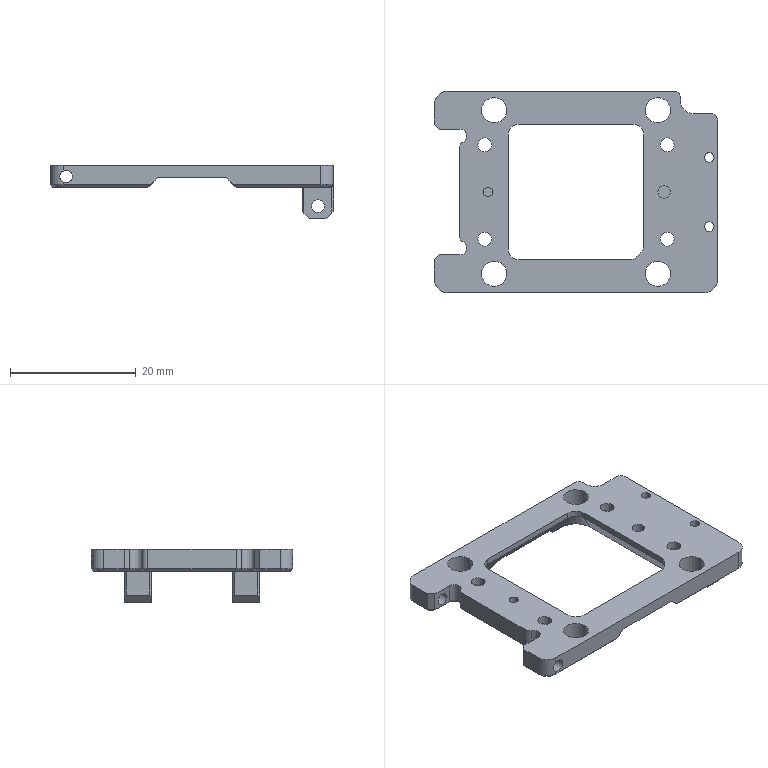NC program | NX | posted with a generic post | part box 45 x 32 x 8.5 mm
Lines 869 to 3036 of 3806, first 1647 of 2162 lines:
(CAVITY_MILL , TOOL : D3)
N1706 T17 M6
N1708 G54
N1710 G17 G0 G90 X18.406 Y16.355 B0. C0. S9500 M3
N1712 G43 Z30. H17
N1714 Z0.722
N1716 G94 G1 Z-0.278 F1100.
N1718 G3 X18.08 Y15.431 R1.
N1720 G2 X18.118 Y15. R2.5
N1722 G1 Y14.437
N1724 G3 X18.618 Y13.937 R0.5
N1726 G1 X19.665
N1728 G3 X20.531 Y14.437 R1.
N1730 G1 X20.589 Y14.537
N1732 Z0.722
N1734 G0 Z30.
N1736 X18.406 Y16.355
N1738 Z0.444
N1740 G1 Z-0.556
N1742 G3 X18.08 Y15.431 R1.
N1744 G2 X18.118 Y15. R2.5
N1746 G1 Y14.437
N1748 G3 X18.618 Y13.937 R0.5
N1750 G1 X19.665
N1752 G3 X20.531 Y14.437 R1.
N1754 G1 X20.589 Y14.537
N1756 Z0.444
N1758 G0 Z30.
N1760 X18.406 Y16.355
N1762 Z0.167
N1764 G1 Z-0.833
N1766 G3 X18.08 Y15.431 R1.
N1768 G2 X18.118 Y15. R2.5
N1770 G1 Y14.437
N1772 G3 X18.618 Y13.937 R0.5
N1774 G1 X19.665
N1776 G3 X20.531 Y14.437 R1.
N1778 G1 X20.589 Y14.537
N1780 Z0.167
N1782 G0 X18.406 Y16.355 Z-0.111
N1784 G1 Z-1.111
N1786 G3 X18.08 Y15.431 R1.
N1788 G2 X18.118 Y15. R2.5
N1790 G1 Y14.437
N1792 G3 X18.618 Y13.937 R0.5
N1794 G1 X19.665
N1796 G3 X20.531 Y14.437 R1.
N1798 G1 X20.589 Y14.537
N1800 Z-0.111
N1802 G0 X18.406 Y16.355 Z-0.389
N1804 G1 Z-1.389
N1806 G3 X18.08 Y15.431 R1.
N1808 G2 X18.118 Y15. R2.5
N1810 G1 Y14.437
N1812 G3 X18.618 Y13.937 R0.5
N1814 G1 X19.665
N1816 G3 X20.531 Y14.437 R1.
N1818 G1 X20.589 Y14.537
N1820 Z-0.389
N1822 G0 X18.406 Y16.355 Z-0.667
N1824 G1 Z-1.667
N1826 G3 X18.08 Y15.431 R1.
N1828 G2 X18.118 Y15. R2.5
N1830 G1 Y14.437
N1832 G3 X18.618 Y13.937 R0.5
N1834 G1 X19.665
N1836 G3 X20.531 Y14.437 R1.
N1838 G1 X20.589 Y14.537
N1840 Z-0.667
N1842 G0 X18.406 Y16.355 Z-0.944
N1844 G1 Z-1.944
N1846 G3 X18.08 Y15.431 R1.
N1848 G2 X18.118 Y15. R2.5
N1850 G1 Y14.437
N1852 G3 X18.618 Y13.937 R0.5
N1854 G1 X19.665
N1856 G3 X20.531 Y14.437 R1.
N1858 G1 X20.589 Y14.537
N1860 Z-0.944
N1862 G0 X18.406 Y16.355 Z-1.222
N1864 G1 Z-2.222
N1866 G3 X18.08 Y15.431 R1.
N1868 G2 X18.118 Y15. R2.5
N1870 G1 Y14.437
N1872 G3 X18.618 Y13.937 R0.5
N1874 G1 X19.665
N1876 G3 X20.531 Y14.437 R1.
N1878 G1 X20.589 Y14.537
N1880 Z-1.222
N1882 G0 X18.406 Y16.355 Z-1.5
N1884 G1 Z-2.5
N1886 G3 X18.08 Y15.431 R1.
N1888 G2 X18.118 Y15. R2.5
N1890 G1 Y14.437
N1892 G3 X18.618 Y13.937 R0.5
N1894 G1 X19.665
N1896 G3 X20.531 Y14.437 R1.
N1898 G1 X20.589 Y14.537
N1900 Z-1.5
N1902 G0 X18.406 Y16.355 Z-1.8
N1904 G1 Z-2.8
N1906 G3 X18.08 Y15.431 R1.
N1908 G2 X18.118 Y15. R2.5
N1910 G1 Y14.437
N1912 G3 X18.618 Y13.937 R0.5
N1914 G1 X19.665
N1916 G3 X20.531 Y14.437 R1.
N1918 G1 X20.589 Y14.537
N1920 Z-1.8
N1922 G0 X18.406 Y16.355 Z-2.1
N1924 G1 Z-3.1
N1926 G3 X18.08 Y15.431 R1.
N1928 G2 X18.118 Y15. R2.5
N1930 G1 Y14.437
N1932 G3 X18.618 Y13.937 R0.5
N1934 G1 X19.665
N1936 G3 X20.531 Y14.437 R1.
N1938 G1 X20.589 Y14.537
N1940 Z-2.1
N1942 G0 X18.402 Y16.362 Z-2.4
N1944 G1 Z-3.4
N1946 G3 X18.079 Y15.437 R1.
N1948 G2 X18.118 Y15. R2.5
N1950 G1 Y14.437
N1952 G3 X18.618 Y13.937 R0.5
N1954 G1 X19.699
N1956 G3 X20.565 Y14.437 R1.
N1958 G1 X20.623 Y14.537
N1960 Z-2.4
N1962 G0 X18.402 Y16.362 Z-2.7
N1964 G1 Z-3.7
N1966 G3 X18.079 Y15.437 R1.
N1968 G2 X18.118 Y15. R2.5
N1970 G1 Y14.437
N1972 G3 X18.618 Y13.937 R0.5
N1974 G1 X19.699
N1976 G3 X20.565 Y14.437 R1.
N1978 G1 X20.623 Y14.537
N1980 Z-2.7
N1982 G0 X18.402 Y16.362 Z-3.
N1984 G1 Z-4.
N1986 G3 X18.079 Y15.437 R1.
N1988 G2 X18.118 Y15. R2.5
N1990 G1 Y14.437
N1992 G3 X18.618 Y13.937 R0.5
N1994 G1 X19.699
N1996 G3 X20.565 Y14.437 R1.
N1998 G1 X20.623 Y14.537
N2000 Z-3.
N2002 G0 X18.402 Y16.362 Z-3.3
N2004 G1 Z-4.3
N2006 G3 X18.079 Y15.437 R1.
N2008 G2 X18.118 Y15. R2.5
N2010 G1 Y14.437
N2012 G3 X18.618 Y13.937 R0.5
N2014 G1 X19.699
N2016 G3 X20.565 Y14.437 R1.
N2018 G1 X20.623 Y14.537
N2020 Z-3.3
N2022 G0 X18.402 Y16.362 Z-3.6
N2024 G1 Z-4.6
N2026 G3 X18.079 Y15.437 R1.
N2028 G2 X18.118 Y15. R2.5
N2030 G1 Y14.437
N2032 G3 X18.618 Y13.937 R0.5
N2034 G1 X19.699
N2036 G3 X20.565 Y14.437 R1.
N2038 G1 X20.623 Y14.537
N2040 Z-3.6
N2042 G0 X18.402 Y16.362 Z-3.9
N2044 G1 Z-4.9
N2046 G3 X18.079 Y15.437 R1.
N2048 G2 X18.118 Y15. R2.5
N2050 G1 Y14.437
N2052 G3 X18.618 Y13.937 R0.5
N2054 G1 X19.699
N2056 G3 X20.565 Y14.437 R1.
N2058 G1 X20.623 Y14.537
N2060 Z-3.9
N2062 G0 X18.402 Y16.362 Z-4.2
N2064 G1 Z-5.2
N2066 G3 X18.079 Y15.437 R1.
N2068 G2 X18.118 Y15. R2.5
N2070 G1 Y14.437
N2072 G3 X18.618 Y13.937 R0.5
N2074 G1 X19.699
N2076 G3 X20.565 Y14.437 R1.
N2078 G1 X20.623 Y14.537
N2080 Z-4.2
N2082 G0 X18.402 Y16.362 Z-4.5
N2084 G1 Z-5.5
N2086 G3 X18.079 Y15.437 R1.
N2088 G2 X18.118 Y15. R2.5
N2090 G1 Y14.437
N2092 G3 X18.618 Y13.937 R0.5
N2094 G1 X19.699
N2096 G3 X20.565 Y14.437 R1.
N2098 G1 X20.623 Y14.537
N2100 Z-4.5
N2102 G0 X18.402 Y16.362 Z-4.8
N2104 G1 Z-5.8
N2106 G3 X18.079 Y15.437 R1.
N2108 G2 X18.118 Y15. R2.5
N2110 G1 Y14.437
N2112 G3 X18.618 Y13.937 R0.5
N2114 G1 X19.699
N2116 G3 X20.565 Y14.437 R1.
N2118 G1 X20.623 Y14.537
N2120 Z-4.8
N2122 G0 X18.402 Y16.362 Z-5.1
N2124 G1 Z-6.1
N2126 G3 X18.079 Y15.437 R1.
N2128 G2 X18.118 Y15. R2.5
N2130 G1 Y14.437
N2132 G3 X18.618 Y13.937 R0.5
N2134 G1 X19.699
N2136 G3 X20.565 Y14.437 R1.
N2138 G1 X20.623 Y14.537
N2140 Z-5.1
N2142 G0 X18.402 Y16.362 Z-5.4
N2144 G1 Z-6.4
N2146 G3 X18.079 Y15.437 R1.
N2148 G2 X18.118 Y15. R2.5
N2150 G1 Y14.437
N2152 G3 X18.618 Y13.937 R0.5
N2154 G1 X19.699
N2156 G3 X20.565 Y14.437 R1.
N2158 G1 X20.623 Y14.537
N2160 Z-5.4
N2162 G0 X18.402 Y16.362 Z-5.7
N2164 G1 Z-6.7
N2166 G3 X18.079 Y15.437 R1.
N2168 G2 X18.118 Y15. R2.5
N2170 G1 Y14.437
N2172 G3 X18.618 Y13.937 R0.5
N2174 G1 X19.699
N2176 G3 X20.565 Y14.437 R1.
N2178 G1 X20.623 Y14.537
N2180 Z-5.7
N2182 G0 X18.402 Y16.362 Z-6.
N2184 G1 Z-7.
N2186 G3 X18.079 Y15.437 R1.
N2188 G2 X18.118 Y15. R2.5
N2190 G1 Y14.437
N2192 G3 X18.618 Y13.937 R0.5
N2194 G1 X19.699
N2196 G3 X20.565 Y14.437 R1.
N2198 G1 X20.623 Y14.537
N2200 Z-6.
N2202 G0 X18.402 Y16.362 Z-6.3
N2204 G1 Z-7.3
N2206 G3 X18.079 Y15.437 R1.
N2208 G2 X18.118 Y15. R2.5
N2210 G1 Y14.437
N2212 G3 X18.618 Y13.937 R0.5
N2214 G1 X19.699
N2216 G3 X20.565 Y14.437 R1.
N2218 G1 X20.623 Y14.537
N2220 Z-6.3
N2222 G0 X18.402 Y16.362 Z-6.6
N2224 G1 Z-7.6
N2226 G3 X18.079 Y15.437 R1.
N2228 G2 X18.118 Y15. R2.5
N2230 G1 Y14.437
N2232 G3 X18.618 Y13.937 R0.5
N2234 G1 X19.699
N2236 G3 X20.565 Y14.437 R1.
N2238 G1 X20.623 Y14.537
N2240 Z-6.6
N2242 G0 X18.402 Y16.362 Z-6.9
N2244 G1 Z-7.9
N2246 G3 X18.079 Y15.437 R1.
N2248 G2 X18.118 Y15. R2.5
N2250 G1 Y14.437
N2252 G3 X18.618 Y13.937 R0.5
N2254 G1 X19.699
N2256 G3 X20.565 Y14.437 R1.
N2258 G1 X20.623 Y14.537
N2260 Z-6.9
N2262 G0 X18.402 Y16.362 Z-7.2
N2264 G1 Z-8.2
N2266 G3 X18.079 Y15.437 R1.
N2268 G2 X18.118 Y15. R2.5
N2270 G1 Y14.437
N2272 G3 X18.618 Y13.937 R0.5
N2274 G1 X19.699
N2276 G3 X20.565 Y14.437 R1.
N2278 G1 X20.623 Y14.537
N2280 Z-7.2
N2282 G0 X18.402 Y16.362 Z-7.5
N2284 G1 Z-8.5
N2286 G3 X18.079 Y15.437 R1.
N2288 G2 X18.118 Y15. R2.5
N2290 G1 Y14.437
N2292 G3 X18.618 Y13.937 R0.5
N2294 G1 X19.699
N2296 G3 X20.565 Y14.437 R1.
N2298 G1 X20.623 Y14.537
N2300 Z-7.5
N2302 G0 Z30.
N2304 X8.7 Y6.805
N2306 Z0.722
N2308 G1 Z-0.278
N2310 X8.8 Y6.862
N2312 G3 X9.3 Y7.728 R1.
N2314 G1 Y9.
N2316 G3 X9. Y9.3 R0.3
N2318 G1 X7.728
N2320 G3 X6.862 Y8.8 R1.
N2322 G1 X6.805 Y8.7
N2324 Z0.722
N2326 G0 Z30.
N2328 X8.7 Y6.805
N2330 Z0.444
N2332 G1 Z-0.556
N2334 X8.8 Y6.862
N2336 G3 X9.3 Y7.728 R1.
N2338 G1 Y9.
N2340 G3 X9. Y9.3 R0.3
N2342 G1 X7.728
N2344 G3 X6.862 Y8.8 R1.
N2346 G1 X6.805 Y8.7
N2348 Z0.444
N2350 G0 Z30.
N2352 X8.7 Y6.805
N2354 Z0.167
N2356 G1 Z-0.833
N2358 X8.8 Y6.862
N2360 G3 X9.3 Y7.728 R1.
N2362 G1 Y9.
N2364 G3 X9. Y9.3 R0.3
N2366 G1 X7.728
N2368 G3 X6.862 Y8.8 R1.
N2370 G1 X6.805 Y8.7
N2372 Z0.167
N2374 G0 X8.7 Y6.806 Z-0.111
N2376 G1 Z-1.111
N2378 X8.8 Y6.864
N2380 G3 X9.3 Y7.73 R1.
N2382 G1 Y9.
N2384 G3 X9. Y9.3 R0.3
N2386 G1 X7.73
N2388 G3 X6.864 Y8.8 R1.
N2390 G1 X6.806 Y8.7
N2392 Z-0.111
N2394 G0 X8.7 Y6.806 Z-0.389
N2396 G1 Z-1.389
N2398 X8.8 Y6.864
N2400 G3 X9.3 Y7.73 R1.
N2402 G1 Y9.
N2404 G3 X9. Y9.3 R0.3
N2406 G1 X7.73
N2408 G3 X6.864 Y8.8 R1.
N2410 G1 X6.806 Y8.7
N2412 Z-0.389
N2414 G0 X8.7 Y6.806 Z-0.667
N2416 G1 Z-1.667
N2418 X8.8 Y6.864
N2420 G3 X9.3 Y7.73 R1.
N2422 G1 Y9.
N2424 G3 X9. Y9.3 R0.3
N2426 G1 X7.73
N2428 G3 X6.864 Y8.8 R1.
N2430 G1 X6.806 Y8.7
N2432 Z-0.667
N2434 G0 X8.7 Y6.806 Z-0.944
N2436 G1 Z-1.944
N2438 X8.8 Y6.864
N2440 G3 X9.3 Y7.73 R1.
N2442 G1 Y9.
N2444 G3 X9. Y9.3 R0.3
N2446 G1 X7.73
N2448 G3 X6.864 Y8.8 R1.
N2450 G1 X6.806 Y8.7
N2452 Z-0.944
N2454 G0 X8.7 Y6.806 Z-1.222
N2456 G1 Z-2.222
N2458 X8.8 Y6.864
N2460 G3 X9.3 Y7.73 R1.
N2462 G1 Y9.
N2464 G3 X9. Y9.3 R0.3
N2466 G1 X7.73
N2468 G3 X6.864 Y8.8 R1.
N2470 G1 X6.806 Y8.7
N2472 Z-1.222
N2474 G0 X8.7 Y6.806 Z-1.5
N2476 G1 Z-2.5
N2478 X8.8 Y6.864
N2480 G3 X9.3 Y7.73 R1.
N2482 G1 Y9.
N2484 G3 X9. Y9.3 R0.3
N2486 G1 X7.73
N2488 G3 X6.864 Y8.8 R1.
N2490 G1 X6.806 Y8.7
N2492 Z-1.5
N2494 G0 X8.7 Y6.806 Z-1.8
N2496 G1 Z-2.8
N2498 X8.8 Y6.864
N2500 G3 X9.3 Y7.73 R1.
N2502 G1 Y9.
N2504 G3 X9. Y9.3 R0.3
N2506 G1 X7.73
N2508 G3 X6.864 Y8.8 R1.
N2510 G1 X6.806 Y8.7
N2512 Z-1.8
N2514 G0 X8.7 Y6.806 Z-2.1
N2516 G1 Z-3.1
N2518 X8.8 Y6.864
N2520 G3 X9.3 Y7.73 R1.
N2522 G1 Y9.
N2524 G3 X9. Y9.3 R0.3
N2526 G1 X7.73
N2528 G3 X6.864 Y8.8 R1.
N2530 G1 X6.806 Y8.7
N2532 Z-2.1
N2534 G0 X8.7 Y6.806 Z-2.4
N2536 G1 Z-3.4
N2538 X8.8 Y6.864
N2540 G3 X9.3 Y7.73 R1.
N2542 G1 Y9.
N2544 G3 X9. Y9.3 R0.3
N2546 G1 X7.73
N2548 G3 X6.864 Y8.8 R1.
N2550 G1 X6.806 Y8.7
N2552 Z-2.4
N2554 G0 X8.7 Y6.806 Z-2.7
N2556 G1 Z-3.7
N2558 X8.8 Y6.864
N2560 G3 X9.3 Y7.73 R1.
N2562 G1 Y9.
N2564 G3 X9. Y9.3 R0.3
N2566 G1 X7.73
N2568 G3 X6.864 Y8.8 R1.
N2570 G1 X6.806 Y8.7
N2572 Z-2.7
N2574 G0 X8.7 Y6.806 Z-3.
N2576 G1 Z-4.
N2578 X8.8 Y6.864
N2580 G3 X9.3 Y7.73 R1.
N2582 G1 Y9.
N2584 G3 X9. Y9.3 R0.3
N2586 G1 X7.73
N2588 G3 X6.864 Y8.8 R1.
N2590 G1 X6.806 Y8.7
N2592 Z-3.
N2594 G0 X8.7 Y6.806 Z-3.3
N2596 G1 Z-4.3
N2598 X8.8 Y6.864
N2600 G3 X9.3 Y7.73 R1.
N2602 G1 Y9.
N2604 G3 X9. Y9.3 R0.3
N2606 G1 X7.73
N2608 G3 X6.864 Y8.8 R1.
N2610 G1 X6.806 Y8.7
N2612 Z-3.3
N2614 G0 X8.7 Y6.806 Z-3.6
N2616 G1 Z-4.6
N2618 X8.8 Y6.864
N2620 G3 X9.3 Y7.73 R1.
N2622 G1 Y9.
N2624 G3 X9. Y9.3 R0.3
N2626 G1 X7.73
N2628 G3 X6.864 Y8.8 R1.
N2630 G1 X6.806 Y8.7
N2632 Z-3.6
N2634 G0 X8.7 Y6.806 Z-3.9
N2636 G1 Z-4.9
N2638 X8.8 Y6.864
N2640 G3 X9.3 Y7.73 R1.
N2642 G1 Y9.
N2644 G3 X9. Y9.3 R0.3
N2646 G1 X7.73
N2648 G3 X6.864 Y8.8 R1.
N2650 G1 X6.806 Y8.7
N2652 Z-3.9
N2654 G0 X8.7 Y6.806 Z-4.2
N2656 G1 Z-5.2
N2658 X8.8 Y6.864
N2660 G3 X9.3 Y7.73 R1.
N2662 G1 Y9.
N2664 G3 X9. Y9.3 R0.3
N2666 G1 X7.73
N2668 G3 X6.864 Y8.8 R1.
N2670 G1 X6.806 Y8.7
N2672 Z-4.2
N2674 G0 X8.7 Y6.806 Z-4.5
N2676 G1 Z-5.5
N2678 X8.8 Y6.864
N2680 G3 X9.3 Y7.73 R1.
N2682 G1 Y9.
N2684 G3 X9. Y9.3 R0.3
N2686 G1 X7.73
N2688 G3 X6.864 Y8.8 R1.
N2690 G1 X6.806 Y8.7
N2692 Z-4.5
N2694 G0 X8.7 Y6.806 Z-4.8
N2696 G1 Z-5.8
N2698 X8.8 Y6.864
N2700 G3 X9.3 Y7.73 R1.
N2702 G1 Y9.
N2704 G3 X9. Y9.3 R0.3
N2706 G1 X7.73
N2708 G3 X6.864 Y8.8 R1.
N2710 G1 X6.806 Y8.7
N2712 Z-4.8
N2714 G0 X8.7 Y6.806 Z-5.1
N2716 G1 Z-6.1
N2718 X8.8 Y6.864
N2720 G3 X9.3 Y7.73 R1.
N2722 G1 Y9.
N2724 G3 X9. Y9.3 R0.3
N2726 G1 X7.73
N2728 G3 X6.864 Y8.8 R1.
N2730 G1 X6.806 Y8.7
N2732 Z-5.1
N2734 G0 X8.7 Y6.806 Z-5.4
N2736 G1 Z-6.4
N2738 X8.8 Y6.864
N2740 G3 X9.3 Y7.73 R1.
N2742 G1 Y9.
N2744 G3 X9. Y9.3 R0.3
N2746 G1 X7.73
N2748 G3 X6.864 Y8.8 R1.
N2750 G1 X6.806 Y8.7
N2752 Z-5.4
N2754 G0 X8.7 Y6.806 Z-5.7
N2756 G1 Z-6.7
N2758 X8.8 Y6.864
N2760 G3 X9.3 Y7.73 R1.
N2762 G1 Y9.
N2764 G3 X9. Y9.3 R0.3
N2766 G1 X7.73
N2768 G3 X6.864 Y8.8 R1.
N2770 G1 X6.806 Y8.7
N2772 Z-5.7
N2774 G0 X8.7 Y6.806 Z-6.
N2776 G1 Z-7.
N2778 X8.8 Y6.864
N2780 G3 X9.3 Y7.73 R1.
N2782 G1 Y9.
N2784 G3 X9. Y9.3 R0.3
N2786 G1 X7.73
N2788 G3 X6.864 Y8.8 R1.
N2790 G1 X6.806 Y8.7
N2792 Z-6.
N2794 G0 X8.7 Y6.806 Z-6.3
N2796 G1 Z-7.3
N2798 X8.8 Y6.864
N2800 G3 X9.3 Y7.73 R1.
N2802 G1 Y9.
N2804 G3 X9. Y9.3 R0.3
N2806 G1 X7.73
N2808 G3 X6.864 Y8.8 R1.
N2810 G1 X6.806 Y8.7
N2812 Z-6.3
N2814 G0 X8.7 Y6.806 Z-6.6
N2816 G1 Z-7.6
N2818 X8.8 Y6.864
N2820 G3 X9.3 Y7.73 R1.
N2822 G1 Y9.
N2824 G3 X9. Y9.3 R0.3
N2826 G1 X7.73
N2828 G3 X6.864 Y8.8 R1.
N2830 G1 X6.806 Y8.7
N2832 Z-6.6
N2834 G0 X8.7 Y6.806 Z-6.9
N2836 G1 Z-7.9
N2838 X8.8 Y6.864
N2840 G3 X9.3 Y7.73 R1.
N2842 G1 Y9.
N2844 G3 X9. Y9.3 R0.3
N2846 G1 X7.73
N2848 G3 X6.864 Y8.8 R1.
N2850 G1 X6.806 Y8.7
N2852 Z-6.9
N2854 G0 X8.7 Y6.806 Z-7.2
N2856 G1 Z-8.2
N2858 X8.8 Y6.864
N2860 G3 X9.3 Y7.73 R1.
N2862 G1 Y9.
N2864 G3 X9. Y9.3 R0.3
N2866 G1 X7.73
N2868 G3 X6.864 Y8.8 R1.
N2870 G1 X6.806 Y8.7
N2872 Z-7.2
N2874 G0 X8.7 Y6.806 Z-7.5
N2876 G1 Z-8.5
N2878 X8.8 Y6.864
N2880 G3 X9.3 Y7.73 R1.
N2882 G1 Y9.
N2884 G3 X9. Y9.3 R0.3
N2886 G1 X7.73
N2888 G3 X6.864 Y8.8 R1.
N2890 G1 X6.806 Y8.7
N2892 Z-7.5
N2894 G0 Z30.
N2896 X6.805 Y-8.7
N2898 Z0.722
N2900 G1 Z-0.278
N2902 X6.862 Y-8.8
N2904 G3 X7.728 Y-9.3 R1.
N2906 G1 X8.379
N2908 G3 X8.591 Y-9.212 R0.3
N2910 G1 X9.212 Y-8.591
N2912 G3 X9.3 Y-8.379 R0.3
N2914 G1 Y-7.728
N2916 G3 X8.8 Y-6.862 R1.
N2918 G1 X8.7 Y-6.805
N2920 Z0.722
N2922 G0 Z30.
N2924 X6.805 Y-8.7
N2926 Z0.444
N2928 G1 Z-0.556
N2930 X6.862 Y-8.8
N2932 G3 X7.728 Y-9.3 R1.
N2934 G1 X8.379
N2936 G3 X8.591 Y-9.212 R0.3
N2938 G1 X9.212 Y-8.591
N2940 G3 X9.3 Y-8.379 R0.3
N2942 G1 Y-7.728
N2944 G3 X8.8 Y-6.862 R1.
N2946 G1 X8.7 Y-6.805
N2948 Z0.444
N2950 G0 Z30.
N2952 X6.805 Y-8.7
N2954 Z0.167
N2956 G1 Z-0.833
N2958 X6.862 Y-8.8
N2960 G3 X7.728 Y-9.3 R1.
N2962 G1 X8.379
N2964 G3 X8.591 Y-9.212 R0.3
N2966 G1 X9.212 Y-8.591
N2968 G3 X9.3 Y-8.379 R0.3
N2970 G1 Y-7.728
N2972 G3 X8.8 Y-6.862 R1.
N2974 G1 X8.7 Y-6.805
N2976 Z0.167
N2978 G0 X6.806 Y-8.7 Z-0.111
N2980 G1 Z-1.111
N2982 X6.864 Y-8.8
N2984 G3 X7.73 Y-9.3 R1.
N2986 G1 X8.379
N2988 G3 X8.591 Y-9.212 R0.3
N2990 G1 X9.212 Y-8.591
N2992 G3 X9.3 Y-8.379 R0.3
N2994 G1 Y-7.73
N2996 G3 X8.8 Y-6.864 R1.
N2998 G1 X8.7 Y-6.806
N3000 Z-0.111
N3002 G0 X6.806 Y-8.7 Z-0.389
N3004 G1 Z-1.389
N3006 X6.864 Y-8.8
N3008 G3 X7.73 Y-9.3 R1.
N3010 G1 X8.379
N3012 G3 X8.591 Y-9.212 R0.3
N3014 G1 X9.212 Y-8.591
N3016 G3 X9.3 Y-8.379 R0.3
N3018 G1 Y-7.73
N3020 G3 X8.8 Y-6.864 R1.
N3022 G1 X8.7 Y-6.806
N3024 Z-0.389
N3026 G0 X6.806 Y-8.7 Z-0.667
N3028 G1 Z-1.667
N3030 X6.864 Y-8.8
N3032 G3 X7.73 Y-9.3 R1.
N3034 G1 X8.379
N3036 G3 X8.591 Y-9.212 R0.3
N3038 G1 X9.212 Y-8.591
N3040 G3 X9.3 Y-8.379 R0.3
N3042 G1 Y-7.73
N3044 G3 X8.8 Y-6.864 R1.
N3046 G1 X8.7 Y-6.806
N3048 Z-0.667
N3050 G0 X6.806 Y-8.7 Z-0.944
N3052 G1 Z-1.944
N3054 X6.864 Y-8.8
N3056 G3 X7.73 Y-9.3 R1.
N3058 G1 X8.379
N3060 G3 X8.591 Y-9.212 R0.3
N3062 G1 X9.212 Y-8.591
N3064 G3 X9.3 Y-8.379 R0.3
N3066 G1 Y-7.73
N3068 G3 X8.8 Y-6.864 R1.
N3070 G1 X8.7 Y-6.806
N3072 Z-0.944
N3074 G0 X6.806 Y-8.7 Z-1.222
N3076 G1 Z-2.222
N3078 X6.864 Y-8.8
N3080 G3 X7.73 Y-9.3 R1.
N3082 G1 X8.379
N3084 G3 X8.591 Y-9.212 R0.3
N3086 G1 X9.212 Y-8.591
N3088 G3 X9.3 Y-8.379 R0.3
N3090 G1 Y-7.73
N3092 G3 X8.8 Y-6.864 R1.
N3094 G1 X8.7 Y-6.806
N3096 Z-1.222
N3098 G0 X6.806 Y-8.7 Z-1.5
N3100 G1 Z-2.5
N3102 X6.864 Y-8.8
N3104 G3 X7.73 Y-9.3 R1.
N3106 G1 X8.379
N3108 G3 X8.591 Y-9.212 R0.3
N3110 G1 X9.212 Y-8.591
N3112 G3 X9.3 Y-8.379 R0.3
N3114 G1 Y-7.73
N3116 G3 X8.8 Y-6.864 R1.
N3118 G1 X8.7 Y-6.806
N3120 Z-1.5
N3122 G0 X6.806 Y-8.7 Z-1.8
N3124 G1 Z-2.8
N3126 X6.864 Y-8.8
N3128 G3 X7.73 Y-9.3 R1.
N3130 G1 X8.379
N3132 G3 X8.591 Y-9.212 R0.3
N3134 G1 X9.212 Y-8.591
N3136 G3 X9.3 Y-8.379 R0.3
N3138 G1 Y-7.73
N3140 G3 X8.8 Y-6.864 R1.
N3142 G1 X8.7 Y-6.806
N3144 Z-1.8
N3146 G0 X6.806 Y-8.7 Z-2.1
N3148 G1 Z-3.1
N3150 X6.864 Y-8.8
N3152 G3 X7.73 Y-9.3 R1.
N3154 G1 X8.379
N3156 G3 X8.591 Y-9.212 R0.3
N3158 G1 X9.212 Y-8.591
N3160 G3 X9.3 Y-8.379 R0.3
N3162 G1 Y-7.73
N3164 G3 X8.8 Y-6.864 R1.
N3166 G1 X8.7 Y-6.806
N3168 Z-2.1
N3170 G0 X6.806 Y-8.7 Z-2.4
N3172 G1 Z-3.4
N3174 X6.864 Y-8.8
N3176 G3 X7.73 Y-9.3 R1.
N3178 G1 X8.379
N3180 G3 X8.591 Y-9.212 R0.3
N3182 G1 X9.212 Y-8.591
N3184 G3 X9.3 Y-8.379 R0.3
N3186 G1 Y-7.73
N3188 G3 X8.8 Y-6.864 R1.
N3190 G1 X8.7 Y-6.806
N3192 Z-2.4
N3194 G0 X6.806 Y-8.7 Z-2.7
N3196 G1 Z-3.7
N3198 X6.864 Y-8.8
N3200 G3 X7.73 Y-9.3 R1.
N3202 G1 X8.379
N3204 G3 X8.591 Y-9.212 R0.3
N3206 G1 X9.212 Y-8.591
N3208 G3 X9.3 Y-8.379 R0.3
N3210 G1 Y-7.73
N3212 G3 X8.8 Y-6.864 R1.
N3214 G1 X8.7 Y-6.806
N3216 Z-2.7
N3218 G0 X6.806 Y-8.7 Z-3.
N3220 G1 Z-4.
N3222 X6.864 Y-8.8
N3224 G3 X7.73 Y-9.3 R1.
N3226 G1 X8.379
N3228 G3 X8.591 Y-9.212 R0.3
N3230 G1 X9.212 Y-8.591
N3232 G3 X9.3 Y-8.379 R0.3
N3234 G1 Y-7.73
N3236 G3 X8.8 Y-6.864 R1.
N3238 G1 X8.7 Y-6.806
N3240 Z-3.
N3242 G0 X6.806 Y-8.7 Z-3.3
N3244 G1 Z-4.3
N3246 X6.864 Y-8.8
N3248 G3 X7.73 Y-9.3 R1.
N3250 G1 X8.379
N3252 G3 X8.591 Y-9.212 R0.3
N3254 G1 X9.212 Y-8.591
N3256 G3 X9.3 Y-8.379 R0.3
N3258 G1 Y-7.73
N3260 G3 X8.8 Y-6.864 R1.
N3262 G1 X8.7 Y-6.806
N3264 Z-3.3
N3266 G0 X6.806 Y-8.7 Z-3.6
N3268 G1 Z-4.6
N3270 X6.864 Y-8.8
N3272 G3 X7.73 Y-9.3 R1.
N3274 G1 X8.379
N3276 G3 X8.591 Y-9.212 R0.3
N3278 G1 X9.212 Y-8.591
N3280 G3 X9.3 Y-8.379 R0.3
N3282 G1 Y-7.73
N3284 G3 X8.8 Y-6.864 R1.
N3286 G1 X8.7 Y-6.806
N3288 Z-3.6
N3290 G0 X6.806 Y-8.7 Z-3.9
N3292 G1 Z-4.9
N3294 X6.864 Y-8.8
N3296 G3 X7.73 Y-9.3 R1.
N3298 G1 X8.379
N3300 G3 X8.591 Y-9.212 R0.3
N3302 G1 X9.212 Y-8.591
N3304 G3 X9.3 Y-8.379 R0.3
N3306 G1 Y-7.73
N3308 G3 X8.8 Y-6.864 R1.
N3310 G1 X8.7 Y-6.806
N3312 Z-3.9
N3314 G0 X6.806 Y-8.7 Z-4.2
N3316 G1 Z-5.2
N3318 X6.864 Y-8.8
N3320 G3 X7.73 Y-9.3 R1.
N3322 G1 X8.379
N3324 G3 X8.591 Y-9.212 R0.3
N3326 G1 X9.212 Y-8.591
N3328 G3 X9.3 Y-8.379 R0.3
N3330 G1 Y-7.73
N3332 G3 X8.8 Y-6.864 R1.
N3334 G1 X8.7 Y-6.806
N3336 Z-4.2
N3338 G0 X6.806 Y-8.7 Z-4.5
N3340 G1 Z-5.5
N3342 X6.864 Y-8.8
N3344 G3 X7.73 Y-9.3 R1.
N3346 G1 X8.379
N3348 G3 X8.591 Y-9.212 R0.3
N3350 G1 X9.212 Y-8.591
N3352 G3 X9.3 Y-8.379 R0.3
N3354 G1 Y-7.73
N3356 G3 X8.8 Y-6.864 R1.
N3358 G1 X8.7 Y-6.806
N3360 Z-4.5
N3362 G0 X6.806 Y-8.7 Z-4.8
N3364 G1 Z-5.8
N3366 X6.864 Y-8.8
N3368 G3 X7.73 Y-9.3 R1.
N3370 G1 X8.379
N3372 G3 X8.591 Y-9.212 R0.3
N3374 G1 X9.212 Y-8.591
N3376 G3 X9.3 Y-8.379 R0.3
N3378 G1 Y-7.73
N3380 G3 X8.8 Y-6.864 R1.
N3382 G1 X8.7 Y-6.806
N3384 Z-4.8
N3386 G0 X6.806 Y-8.7 Z-5.1
N3388 G1 Z-6.1
N3390 X6.864 Y-8.8
N3392 G3 X7.73 Y-9.3 R1.
N3394 G1 X8.379
N3396 G3 X8.591 Y-9.212 R0.3
N3398 G1 X9.212 Y-8.591
N3400 G3 X9.3 Y-8.379 R0.3
N3402 G1 Y-7.73
N3404 G3 X8.8 Y-6.864 R1.
N3406 G1 X8.7 Y-6.806
N3408 Z-5.1
N3410 G0 X6.806 Y-8.7 Z-5.4
N3412 G1 Z-6.4
N3414 X6.864 Y-8.8
N3416 G3 X7.73 Y-9.3 R1.
N3418 G1 X8.379
N3420 G3 X8.591 Y-9.212 R0.3
N3422 G1 X9.212 Y-8.591
N3424 G3 X9.3 Y-8.379 R0.3
N3426 G1 Y-7.73
N3428 G3 X8.8 Y-6.864 R1.
N3430 G1 X8.7 Y-6.806
N3432 Z-5.4
N3434 G0 X6.806 Y-8.7 Z-5.7
N3436 G1 Z-6.7
N3438 X6.864 Y-8.8
N3440 G3 X7.73 Y-9.3 R1.
N3442 G1 X8.379
N3444 G3 X8.591 Y-9.212 R0.3
N3446 G1 X9.212 Y-8.591
N3448 G3 X9.3 Y-8.379 R0.3
N3450 G1 Y-7.73
N3452 G3 X8.8 Y-6.864 R1.
N3454 G1 X8.7 Y-6.806
N3456 Z-5.7
N3458 G0 X6.806 Y-8.7 Z-6.
N3460 G1 Z-7.
N3462 X6.864 Y-8.8
N3464 G3 X7.73 Y-9.3 R1.
N3466 G1 X8.379
N3468 G3 X8.591 Y-9.212 R0.3
N3470 G1 X9.212 Y-8.591
N3472 G3 X9.3 Y-8.379 R0.3
N3474 G1 Y-7.73
N3476 G3 X8.8 Y-6.864 R1.
N3478 G1 X8.7 Y-6.806
N3480 Z-6.
N3482 G0 X6.806 Y-8.7 Z-6.3
N3484 G1 Z-7.3
N3486 X6.864 Y-8.8
N3488 G3 X7.73 Y-9.3 R1.
N3490 G1 X8.379
N3492 G3 X8.591 Y-9.212 R0.3
N3494 G1 X9.212 Y-8.591
N3496 G3 X9.3 Y-8.379 R0.3
N3498 G1 Y-7.73
N3500 G3 X8.8 Y-6.864 R1.
N3502 G1 X8.7 Y-6.806
N3504 Z-6.3
N3506 G0 X6.806 Y-8.7 Z-6.6
N3508 G1 Z-7.6
N3510 X6.864 Y-8.8
N3512 G3 X7.73 Y-9.3 R1.
N3514 G1 X8.379
N3516 G3 X8.591 Y-9.212 R0.3
N3518 G1 X9.212 Y-8.591
N3520 G3 X9.3 Y-8.379 R0.3
N3522 G1 Y-7.73
N3524 G3 X8.8 Y-6.864 R1.
N3526 G1 X8.7 Y-6.806
N3528 Z-6.6
N3530 G0 X6.806 Y-8.7 Z-6.9
N3532 G1 Z-7.9
N3534 X6.864 Y-8.8
N3536 G3 X7.73 Y-9.3 R1.
N3538 G1 X8.379
N3540 G3 X8.591 Y-9.212 R0.3
N3542 G1 X9.212 Y-8.591
N3544 G3 X9.3 Y-8.379 R0.3
N3546 G1 Y-7.73
N3548 G3 X8.8 Y-6.864 R1.
N3550 G1 X8.7 Y-6.806
N3552 Z-6.9
N3554 G0 X6.806 Y-8.7 Z-7.2
N3556 G1 Z-8.2
N3558 X6.864 Y-8.8
N3560 G3 X7.73 Y-9.3 R1.
N3562 G1 X8.379
N3564 G3 X8.591 Y-9.212 R0.3
N3566 G1 X9.212 Y-8.591
N3568 G3 X9.3 Y-8.379 R0.3
N3570 G1 Y-7.73
N3572 G3 X8.8 Y-6.864 R1.
N3574 G1 X8.7 Y-6.806
N3576 Z-7.2
N3578 G0 X6.806 Y-8.7 Z-7.5
N3580 G1 Z-8.5
N3582 X6.864 Y-8.8
N3584 G3 X7.73 Y-9.3 R1.
N3586 G1 X8.379
N3588 G3 X8.591 Y-9.212 R0.3
N3590 G1 X9.212 Y-8.591
N3592 G3 X9.3 Y-8.379 R0.3
N3594 G1 Y-7.73
N3596 G3 X8.8 Y-6.864 R1.
N3598 G1 X8.7 Y-6.806
N3600 Z-7.5
N3602 G0 Z30.
N3604 X-8.7 Y-6.805
N3606 Z0.722
N3608 G1 Z-0.278
N3610 X-8.8 Y-6.862
N3612 G3 X-9.3 Y-7.728 R1.
N3614 G1 Y-9.
N3616 G3 X-9. Y-9.3 R0.3
N3618 G1 X-7.728
N3620 G3 X-6.862 Y-8.8 R1.
N3622 G1 X-6.805 Y-8.7
N3624 Z0.722
N3626 G0 Z30.
N3628 X-8.7 Y-6.805
N3630 Z0.444
N3632 G1 Z-0.556
N3634 X-8.8 Y-6.862
N3636 G3 X-9.3 Y-7.728 R1.
N3638 G1 Y-9.
N3640 G3 X-9. Y-9.3 R0.3
N3642 G1 X-7.728
N3644 G3 X-6.862 Y-8.8 R1.
N3646 G1 X-6.805 Y-8.7
N3648 Z0.444
N3650 G0 Z30.
N3652 X-8.7 Y-6.805
N3654 Z0.167
N3656 G1 Z-0.833
N3658 X-8.8 Y-6.862
N3660 G3 X-9.3 Y-7.728 R1.
N3662 G1 Y-9.
N3664 G3 X-9. Y-9.3 R0.3
N3666 G1 X-7.728
N3668 G3 X-6.862 Y-8.8 R1.
N3670 G1 X-6.805 Y-8.7
N3672 Z0.167
N3674 G0 X-8.7 Y-6.806 Z-0.111
N3676 G1 Z-1.111
N3678 X-8.8 Y-6.864
N3680 G3 X-9.3 Y-7.73 R1.
N3682 G1 Y-9.
N3684 G3 X-9. Y-9.3 R0.3
N3686 G1 X-7.73
N3688 G3 X-6.864 Y-8.8 R1.
N3690 G1 X-6.806 Y-8.7
N3692 Z-0.111
N3694 G0 X-8.7 Y-6.806 Z-0.389
N3696 G1 Z-1.389
N3698 X-8.8 Y-6.864
N3700 G3 X-9.3 Y-7.73 R1.
N3702 G1 Y-9.
N3704 G3 X-9. Y-9.3 R0.3
N3706 G1 X-7.73
N3708 G3 X-6.864 Y-8.8 R1.
N3710 G1 X-6.806 Y-8.7
N3712 Z-0.389
N3714 G0 X-8.7 Y-6.806 Z-0.667
N3716 G1 Z-1.667
N3718 X-8.8 Y-6.864
N3720 G3 X-9.3 Y-7.73 R1.
N3722 G1 Y-9.
N3724 G3 X-9. Y-9.3 R0.3
N3726 G1 X-7.73
N3728 G3 X-6.864 Y-8.8 R1.
N3730 G1 X-6.806 Y-8.7
N3732 Z-0.667
N3734 G0 X-8.7 Y-6.806 Z-0.944
N3736 G1 Z-1.944
N3738 X-8.8 Y-6.864
N3740 G3 X-9.3 Y-7.73 R1.
N3742 G1 Y-9.
N3744 G3 X-9. Y-9.3 R0.3
N3746 G1 X-7.73
N3748 G3 X-6.864 Y-8.8 R1.
N3750 G1 X-6.806 Y-8.7
N3752 Z-0.944
N3754 G0 X-8.7 Y-6.806 Z-1.222
N3756 G1 Z-2.222
N3758 X-8.8 Y-6.864
N3760 G3 X-9.3 Y-7.73 R1.
N3762 G1 Y-9.
N3764 G3 X-9. Y-9.3 R0.3
N3766 G1 X-7.73
N3768 G3 X-6.864 Y-8.8 R1.
N3770 G1 X-6.806 Y-8.7
N3772 Z-1.222
N3774 G0 X-8.7 Y-6.806 Z-1.5
N3776 G1 Z-2.5
N3778 X-8.8 Y-6.864
N3780 G3 X-9.3 Y-7.73 R1.
N3782 G1 Y-9.
N3784 G3 X-9. Y-9.3 R0.3
N3786 G1 X-7.73
N3788 G3 X-6.864 Y-8.8 R1.
N3790 G1 X-6.806 Y-8.7
N3792 Z-1.5
N3794 G0 X-8.7 Y-6.806 Z-1.8
N3796 G1 Z-2.8
N3798 X-8.8 Y-6.864
N3800 G3 X-9.3 Y-7.73 R1.
N3802 G1 Y-9.
N3804 G3 X-9. Y-9.3 R0.3
N3806 G1 X-7.73
N3808 G3 X-6.864 Y-8.8 R1.
N3810 G1 X-6.806 Y-8.7
N3812 Z-1.8
N3814 G0 X-8.7 Y-6.806 Z-2.1
N3816 G1 Z-3.1
N3818 X-8.8 Y-6.864
N3820 G3 X-9.3 Y-7.73 R1.
N3822 G1 Y-9.
N3824 G3 X-9. Y-9.3 R0.3
N3826 G1 X-7.73
N3828 G3 X-6.864 Y-8.8 R1.
N3830 G1 X-6.806 Y-8.7
N3832 Z-2.1
N3834 G0 X-8.7 Y-6.806 Z-2.4
N3836 G1 Z-3.4
N3838 X-8.8 Y-6.864
N3840 G3 X-9.3 Y-7.73 R1.
N3842 G1 Y-9.
N3844 G3 X-9. Y-9.3 R0.3
N3846 G1 X-7.73
N3848 G3 X-6.864 Y-8.8 R1.
N3850 G1 X-6.806 Y-8.7
N3852 Z-2.4
N3854 G0 X-8.7 Y-6.806 Z-2.7
N3856 G1 Z-3.7
N3858 X-8.8 Y-6.864
N3860 G3 X-9.3 Y-7.73 R1.
N3862 G1 Y-9.
N3864 G3 X-9. Y-9.3 R0.3
N3866 G1 X-7.73
N3868 G3 X-6.864 Y-8.8 R1.
N3870 G1 X-6.806 Y-8.7
N3872 Z-2.7
N3874 G0 X-8.7 Y-6.806 Z-3.
N3876 G1 Z-4.
N3878 X-8.8 Y-6.864
N3880 G3 X-9.3 Y-7.73 R1.
N3882 G1 Y-9.
N3884 G3 X-9. Y-9.3 R0.3
N3886 G1 X-7.73
N3888 G3 X-6.864 Y-8.8 R1.
N3890 G1 X-6.806 Y-8.7
N3892 Z-3.
N3894 G0 X-8.7 Y-6.806 Z-3.3
N3896 G1 Z-4.3
N3898 X-8.8 Y-6.864
N3900 G3 X-9.3 Y-7.73 R1.
N3902 G1 Y-9.
N3904 G3 X-9. Y-9.3 R0.3
N3906 G1 X-7.73
N3908 G3 X-6.864 Y-8.8 R1.
N3910 G1 X-6.806 Y-8.7
N3912 Z-3.3
N3914 G0 X-8.7 Y-6.806 Z-3.6
N3916 G1 Z-4.6
N3918 X-8.8 Y-6.864
N3920 G3 X-9.3 Y-7.73 R1.
N3922 G1 Y-9.
N3924 G3 X-9. Y-9.3 R0.3
N3926 G1 X-7.73
N3928 G3 X-6.864 Y-8.8 R1.
N3930 G1 X-6.806 Y-8.7
N3932 Z-3.6
N3934 G0 X-8.7 Y-6.806 Z-3.9
N3936 G1 Z-4.9
N3938 X-8.8 Y-6.864
N3940 G3 X-9.3 Y-7.73 R1.
N3942 G1 Y-9.
N3944 G3 X-9. Y-9.3 R0.3
N3946 G1 X-7.73
N3948 G3 X-6.864 Y-8.8 R1.
N3950 G1 X-6.806 Y-8.7
N3952 Z-3.9
N3954 G0 X-8.7 Y-6.806 Z-4.2
N3956 G1 Z-5.2
N3958 X-8.8 Y-6.864
N3960 G3 X-9.3 Y-7.73 R1.
N3962 G1 Y-9.
N3964 G3 X-9. Y-9.3 R0.3
N3966 G1 X-7.73
N3968 G3 X-6.864 Y-8.8 R1.
N3970 G1 X-6.806 Y-8.7
N3972 Z-4.2
N3974 G0 X-8.7 Y-6.806 Z-4.5
N3976 G1 Z-5.5
N3978 X-8.8 Y-6.864
N3980 G3 X-9.3 Y-7.73 R1.
N3982 G1 Y-9.
N3984 G3 X-9. Y-9.3 R0.3
N3986 G1 X-7.73
N3988 G3 X-6.864 Y-8.8 R1.
N3990 G1 X-6.806 Y-8.7
N3992 Z-4.5
N3994 G0 X-8.7 Y-6.806 Z-4.8
N3996 G1 Z-5.8
N3998 X-8.8 Y-6.864
N4000 G3 X-9.3 Y-7.73 R1.
N4002 G1 Y-9.
N4004 G3 X-9. Y-9.3 R0.3
N4006 G1 X-7.73
N4008 G3 X-6.864 Y-8.8 R1.
N4010 G1 X-6.806 Y-8.7
N4012 Z-4.8
N4014 G0 X-8.7 Y-6.806 Z-5.1
N4016 G1 Z-6.1
N4018 X-8.8 Y-6.864
N4020 G3 X-9.3 Y-7.73 R1.
N4022 G1 Y-9.
N4024 G3 X-9. Y-9.3 R0.3
N4026 G1 X-7.73
N4028 G3 X-6.864 Y-8.8 R1.
N4030 G1 X-6.806 Y-8.7
N4032 Z-5.1
N4034 G0 X-8.7 Y-6.806 Z-5.4
N4036 G1 Z-6.4
N4038 X-8.8 Y-6.864
N4040 G3 X-9.3 Y-7.73 R1.
N4042 G1 Y-9.
N4044 G3 X-9. Y-9.3 R0.3
N4046 G1 X-7.73
N4048 G3 X-6.864 Y-8.8 R1.
N4050 G1 X-6.806 Y-8.7
N4052 Z-5.4
N4054 G0 X-8.7 Y-6.806 Z-5.7
N4056 G1 Z-6.7
N4058 X-8.8 Y-6.864
N4060 G3 X-9.3 Y-7.73 R1.
N4062 G1 Y-9.
N4064 G3 X-9. Y-9.3 R0.3
N4066 G1 X-7.73
N4068 G3 X-6.864 Y-8.8 R1.
N4070 G1 X-6.806 Y-8.7
N4072 Z-5.7
N4074 G0 X-8.7 Y-6.806 Z-6.
N4076 G1 Z-7.
N4078 X-8.8 Y-6.864
N4080 G3 X-9.3 Y-7.73 R1.
N4082 G1 Y-9.
N4084 G3 X-9. Y-9.3 R0.3
N4086 G1 X-7.73
N4088 G3 X-6.864 Y-8.8 R1.
N4090 G1 X-6.806 Y-8.7
N4092 Z-6.
N4094 G0 X-8.7 Y-6.806 Z-6.3
N4096 G1 Z-7.3
N4098 X-8.8 Y-6.864
N4100 G3 X-9.3 Y-7.73 R1.
N4102 G1 Y-9.
N4104 G3 X-9. Y-9.3 R0.3
N4106 G1 X-7.73
N4108 G3 X-6.864 Y-8.8 R1.
N4110 G1 X-6.806 Y-8.7
N4112 Z-6.3
N4114 G0 X-8.7 Y-6.806 Z-6.6
N4116 G1 Z-7.6
N4118 X-8.8 Y-6.864
N4120 G3 X-9.3 Y-7.73 R1.
N4122 G1 Y-9.
N4124 G3 X-9. Y-9.3 R0.3
N4126 G1 X-7.73
N4128 G3 X-6.864 Y-8.8 R1.
N4130 G1 X-6.806 Y-8.7
N4132 Z-6.6
N4134 G0 X-8.7 Y-6.806 Z-6.9
N4136 G1 Z-7.9
N4138 X-8.8 Y-6.864
N4140 G3 X-9.3 Y-7.73 R1.
N4142 G1 Y-9.
N4144 G3 X-9. Y-9.3 R0.3
N4146 G1 X-7.73
N4148 G3 X-6.864 Y-8.8 R1.
N4150 G1 X-6.806 Y-8.7
N4152 Z-6.9
N4154 G0 X-8.7 Y-6.806 Z-7.2
N4156 G1 Z-8.2
N4158 X-8.8 Y-6.864
N4160 G3 X-9.3 Y-7.73 R1.
N4162 G1 Y-9.
N4164 G3 X-9. Y-9.3 R0.3
N4166 G1 X-7.73
N4168 G3 X-6.864 Y-8.8 R1.
N4170 G1 X-6.806 Y-8.7
N4172 Z-7.2
N4174 G0 X-8.7 Y-6.806 Z-7.5
N4176 G1 Z-8.5
N4178 X-8.8 Y-6.864
N4180 G3 X-9.3 Y-7.73 R1.
N4182 G1 Y-9.
N4184 G3 X-9. Y-9.3 R0.3
N4186 G1 X-7.73
N4188 G3 X-6.864 Y-8.8 R1.
N4190 G1 X-6.806 Y-8.7
N4192 Z-7.5
N4194 G0 Z30.
N4196 X-22.421 Y-8.028
N4198 Z0.722
N4200 G1 Z-0.278
N4202 G3 X-21.572 Y-8.5 R1.
N4204 G1 X-19.539
N4206 G2 X-20. Y-7.053 R2.5
N4208 G1 Y-6.858
N4210 G3 X-20.5 Y-5.992 R1.
N4212 G1 X-20.6 Y-5.934
N4214 Z0.722
N4216 G0 Z30.
N4218 X-22.421 Y-8.028
N4220 Z0.444
N4222 G1 Z-0.556
N4224 G3 X-21.572 Y-8.5 R1.
N4226 G1 X-19.539
N4228 G2 X-20. Y-7.053 R2.5
N4230 G1 Y-6.858
N4232 G3 X-20.5 Y-5.992 R1.
N4234 G1 X-20.6 Y-5.934
N4236 Z0.444
N4238 G0 Z30.
N4240 X-22.421 Y-8.028
N4242 Z0.167
N4244 G1 Z-0.833
N4246 G3 X-21.572 Y-8.5 R1.
N4248 G1 X-19.539
N4250 G2 X-20. Y-7.053 R2.5
N4252 G1 Y-6.858
N4254 G3 X-20.5 Y-5.992 R1.
N4256 G1 X-20.6 Y-5.934
N4258 Z0.167
N4260 G0 X-22.421 Y-8.028 Z-0.111
N4262 G1 Z-1.111
N4264 G3 X-21.572 Y-8.5 R1.
N4266 G1 X-19.539
N4268 G2 X-20. Y-7.053 R2.5
N4270 G1 Y-6.858
N4272 G3 X-20.5 Y-5.992 R1.
N4274 G1 X-20.6 Y-5.934
N4276 Z-0.111
N4278 G0 X-22.421 Y-8.028 Z-0.389
N4280 G1 Z-1.389
N4282 G3 X-21.572 Y-8.5 R1.
N4284 G1 X-19.539
N4286 G2 X-20. Y-7.053 R2.5
N4288 G1 Y-6.858
N4290 G3 X-20.5 Y-5.992 R1.
N4292 G1 X-20.6 Y-5.934
N4294 Z-0.389
N4296 G0 X-22.421 Y-8.028 Z-0.667
N4298 G1 Z-1.667
N4300 G3 X-21.572 Y-8.5 R1.
N4302 G1 X-19.539
N4304 G2 X-20. Y-7.053 R2.5
N4306 G1 Y-6.858
N4308 G3 X-20.5 Y-5.992 R1.
N4310 G1 X-20.6 Y-5.934
N4312 Z-0.667
N4314 G0 X-22.421 Y-8.028 Z-0.944
N4316 G1 Z-1.944
N4318 G3 X-21.572 Y-8.5 R1.
N4320 G1 X-19.539
N4322 G2 X-20. Y-7.053 R2.5
N4324 G1 Y-6.858
N4326 G3 X-20.5 Y-5.992 R1.
N4328 G1 X-20.6 Y-5.934
N4330 Z-0.944
N4332 G0 X-22.421 Y-8.028 Z-1.222
N4334 G1 Z-2.222
N4336 G3 X-21.572 Y-8.5 R1.
N4338 G1 X-19.539
N4340 G2 X-20. Y-7.053 R2.5
N4342 G1 Y-6.858
N4344 G3 X-20.5 Y-5.992 R1.
N4346 G1 X-20.6 Y-5.934
N4348 Z-1.222
N4350 G0 X-22.421 Y-8.028 Z-1.5
N4352 G1 Z-2.5
N4354 G3 X-21.572 Y-8.5 R1.
N4356 G1 X-19.539
N4358 G2 X-20. Y-7.053 R2.5
N4360 G1 Y-6.858
N4362 G3 X-20.5 Y-5.992 R1.
N4364 G1 X-20.6 Y-5.934
N4366 Z-1.5
N4368 G0 X-22.421 Y-8.028 Z-1.8
N4370 G1 Z-2.8
N4372 G3 X-21.572 Y-8.5 R1.
N4374 G1 X-19.539
N4376 G2 X-20. Y-7.053 R2.5
N4378 G1 Y-6.858
N4380 G3 X-20.5 Y-5.992 R1.
N4382 G1 X-20.6 Y-5.934
N4384 Z-1.8
N4386 G0 X-22.421 Y-8.028 Z-2.1
N4388 G1 Z-3.1
N4390 G3 X-21.571 Y-8.5 R1.
N4392 G1 X-19.539
N4394 G2 X-20. Y-7.053 R2.5
N4396 G1 Y-6.859
N4398 G3 X-20.5 Y-5.993 R1.
N4400 G1 X-20.6 Y-5.935
N4402 Z-2.1
N4404 G0 X-22.432 Y-8.032 Z-2.4
N4406 G1 Z-3.4
N4408 G3 X-21.586 Y-8.5 R1.
N4410 G1 X-19.539
N4412 G2 X-20. Y-7.053 R2.5
N4414 G1 Y-6.841
N4416 G3 X-20.5 Y-5.975 R1.
N4418 G1 X-20.6 Y-5.917
N4420 Z-2.4
N4422 G0 X-22.432 Y-8.032 Z-2.7
N4424 G1 Z-3.7
N4426 G3 X-21.586 Y-8.5 R1.
N4428 G1 X-19.539
N4430 G2 X-20. Y-7.053 R2.5
N4432 G1 Y-6.841
N4434 G3 X-20.5 Y-5.975 R1.
N4436 G1 X-20.6 Y-5.917
N4438 Z-2.7
N4440 G0 X-22.432 Y-8.032 Z-3.
N4442 G1 Z-4.
N4444 G3 X-21.586 Y-8.5 R1.
N4446 G1 X-19.539
N4448 G2 X-20. Y-7.053 R2.5
N4450 G1 Y-6.841
N4452 G3 X-20.5 Y-5.975 R1.
N4454 G1 X-20.6 Y-5.917
N4456 Z-3.
N4458 G0 X-22.432 Y-8.032 Z-3.3
N4460 G1 Z-4.3
N4462 G3 X-21.586 Y-8.5 R1.
N4464 G1 X-19.539
N4466 G2 X-20. Y-7.053 R2.5
N4468 G1 Y-6.841
N4470 G3 X-20.5 Y-5.975 R1.
N4472 G1 X-20.6 Y-5.917
N4474 Z-3.3
N4476 G0 X-22.432 Y-8.032 Z-3.6
N4478 G1 Z-4.6
N4480 G3 X-21.586 Y-8.5 R1.
N4482 G1 X-19.539
N4484 G2 X-20. Y-7.053 R2.5
N4486 G1 Y-6.841
N4488 G3 X-20.5 Y-5.975 R1.
N4490 G1 X-20.6 Y-5.917
N4492 Z-3.6
N4494 G0 X-22.432 Y-8.032 Z-3.9
N4496 G1 Z-4.9
N4498 G3 X-21.586 Y-8.5 R1.
N4500 G1 X-19.539
N4502 G2 X-20. Y-7.053 R2.5
N4504 G1 Y-6.841
N4506 G3 X-20.5 Y-5.975 R1.
N4508 G1 X-20.6 Y-5.917
N4510 Z-3.9
N4512 G0 X-22.432 Y-8.032 Z-4.2
N4514 G1 Z-5.2
N4516 G3 X-21.586 Y-8.5 R1.
N4518 G1 X-19.539
N4520 G2 X-20. Y-7.053 R2.5
N4522 G1 Y-6.841
N4524 G3 X-20.5 Y-5.975 R1.
N4526 G1 X-20.6 Y-5.917
N4528 Z-4.2
N4530 G0 X-22.432 Y-8.032 Z-4.5
N4532 G1 Z-5.5
N4534 G3 X-21.586 Y-8.5 R1.
N4536 G1 X-19.539
N4538 G2 X-20. Y-7.053 R2.5
N4540 G1 Y-6.841
N4542 G3 X-20.5 Y-5.975 R1.
N4544 G1 X-20.6 Y-5.917
N4546 Z-4.5
N4548 G0 X-22.432 Y-8.032 Z-4.8
N4550 G1 Z-5.8
N4552 G3 X-21.586 Y-8.5 R1.
N4554 G1 X-19.539
N4556 G2 X-20. Y-7.053 R2.5
N4558 G1 Y-6.841
N4560 G3 X-20.5 Y-5.975 R1.
N4562 G1 X-20.6 Y-5.917
N4564 Z-4.8
N4566 G0 X-22.432 Y-8.032 Z-5.1
N4568 G1 Z-6.1
N4570 G3 X-21.586 Y-8.5 R1.
N4572 G1 X-19.539
N4574 G2 X-20. Y-7.053 R2.5
N4576 G1 Y-6.841
N4578 G3 X-20.5 Y-5.975 R1.
N4580 G1 X-20.6 Y-5.917
N4582 Z-5.1
N4584 G0 X-22.432 Y-8.032 Z-5.4
N4586 G1 Z-6.4
N4588 G3 X-21.586 Y-8.5 R1.
N4590 G1 X-19.539
N4592 G2 X-20. Y-7.053 R2.5
N4594 G1 Y-6.841
N4596 G3 X-20.5 Y-5.975 R1.
N4598 G1 X-20.6 Y-5.917
N4600 Z-5.4
N4602 G0 X-22.432 Y-8.032 Z-5.7
N4604 G1 Z-6.7
N4606 G3 X-21.586 Y-8.5 R1.
N4608 G1 X-19.539
N4610 G2 X-20. Y-7.053 R2.5
N4612 G1 Y-6.841
N4614 G3 X-20.5 Y-5.975 R1.
N4616 G1 X-20.6 Y-5.917
N4618 Z-5.7
N4620 G0 X-22.432 Y-8.032 Z-6.
N4622 G1 Z-7.
N4624 G3 X-21.586 Y-8.5 R1.
N4626 G1 X-19.539
N4628 G2 X-20. Y-7.053 R2.5
N4630 G1 Y-6.841
N4632 G3 X-20.5 Y-5.975 R1.
N4634 G1 X-20.6 Y-5.917
N4636 Z-6.
N4638 G0 X-22.432 Y-8.032 Z-6.3
N4640 G1 Z-7.3
N4642 G3 X-21.586 Y-8.5 R1.
N4644 G1 X-19.539
N4646 G2 X-20. Y-7.053 R2.5
N4648 G1 Y-6.841
N4650 G3 X-20.5 Y-5.975 R1.
N4652 G1 X-20.6 Y-5.917
N4654 Z-6.3
N4656 G0 X-22.432 Y-8.032 Z-6.6
N4658 G1 Z-7.6
N4660 G3 X-21.586 Y-8.5 R1.
N4662 G1 X-19.539
N4664 G2 X-20. Y-7.053 R2.5
N4666 G1 Y-6.841
N4668 G3 X-20.5 Y-5.975 R1.
N4670 G1 X-20.6 Y-5.917
N4672 Z-6.6
N4674 G0 X-22.432 Y-8.032 Z-6.9
N4676 G1 Z-7.9
N4678 G3 X-21.586 Y-8.5 R1.
N4680 G1 X-19.539
N4682 G2 X-20. Y-7.053 R2.5
N4684 G1 Y-6.841
N4686 G3 X-20.5 Y-5.975 R1.
N4688 G1 X-20.6 Y-5.917
N4690 Z-6.9
N4692 G0 X-22.432 Y-8.032 Z-7.2
N4694 G1 Z-8.2
N4696 G3 X-21.586 Y-8.5 R1.
N4698 G1 X-19.539
N4700 G2 X-20. Y-7.053 R2.5
N4702 G1 Y-6.841
N4704 G3 X-20.5 Y-5.975 R1.
N4706 G1 X-20.6 Y-5.917
N4708 Z-7.2
N4710 G0 X-22.432 Y-8.032 Z-7.5
N4712 G1 Z-8.5
N4714 G3 X-21.586 Y-8.5 R1.
N4716 G1 X-19.539
N4718 G2 X-20. Y-7.053 R2.5
N4720 G1 Y-6.841
N4722 G3 X-20.5 Y-5.975 R1.
N4724 G1 X-20.6 Y-5.917
N4726 Z-7.5
N4728 G0 Z30.
N4730 Y5.934
N4732 Z0.722
N4734 G1 Z-0.278
N4736 X-20.5 Y5.992
N4738 G3 X-20. Y6.858 R1.
N4740 G1 Y7.053
N4742 G2 X-19.539 Y8.5 R2.5
N4744 G1 X-21.572
N4746 G3 X-22.421 Y8.028 R1.
N4748 G1 Z0.722
N4750 G0 Z30.
N4752 X-20.6 Y5.934
N4754 Z0.444
N4756 G1 Z-0.556
N4758 X-20.5 Y5.992
N4760 G3 X-20. Y6.858 R1.
N4762 G1 Y7.053
N4764 G2 X-19.539 Y8.5 R2.5
N4766 G1 X-21.572
N4768 G3 X-22.421 Y8.028 R1.
N4770 G1 Z0.444
N4772 G0 Z30.
N4774 X-20.6 Y5.934
N4776 Z0.167
N4778 G1 Z-0.833
N4780 X-20.5 Y5.992
N4782 G3 X-20. Y6.858 R1.
N4784 G1 Y7.053
N4786 G2 X-19.539 Y8.5 R2.5
N4788 G1 X-21.572
N4790 G3 X-22.421 Y8.028 R1.
N4792 G1 Z0.167
N4794 G0 X-20.6 Y5.934 Z-0.111
N4796 G1 Z-1.111
N4798 X-20.5 Y5.992
N4800 G3 X-20. Y6.858 R1.
N4802 G1 Y7.053
N4804 G2 X-19.539 Y8.5 R2.5
N4806 G1 X-21.572
N4808 G3 X-22.421 Y8.028 R1.
N4810 G1 Z-0.111
N4812 G0 X-20.6 Y5.934 Z-0.389
N4814 G1 Z-1.389
N4816 X-20.5 Y5.992
N4818 G3 X-20. Y6.858 R1.
N4820 G1 Y7.053
N4822 G2 X-19.539 Y8.5 R2.5
N4824 G1 X-21.572
N4826 G3 X-22.421 Y8.028 R1.
N4828 G1 Z-0.389
N4830 G0 X-20.6 Y5.934 Z-0.667
N4832 G1 Z-1.667
N4834 X-20.5 Y5.992
N4836 G3 X-20. Y6.858 R1.
N4838 G1 Y7.053
N4840 G2 X-19.539 Y8.5 R2.5
N4842 G1 X-21.572
N4844 G3 X-22.421 Y8.028 R1.
N4846 G1 Z-0.667
N4848 G0 X-20.6 Y5.934 Z-0.944
N4850 G1 Z-1.944
N4852 X-20.5 Y5.992
N4854 G3 X-20. Y6.858 R1.
N4856 G1 Y7.053
N4858 G2 X-19.539 Y8.5 R2.5
N4860 G1 X-21.572
N4862 G3 X-22.421 Y8.028 R1.
N4864 G1 Z-0.944
N4866 G0 X-20.6 Y5.934 Z-1.222
N4868 G1 Z-2.222
N4870 X-20.5 Y5.992
N4872 G3 X-20. Y6.858 R1.
N4874 G1 Y7.053
N4876 G2 X-19.539 Y8.5 R2.5
N4878 G1 X-21.572
N4880 G3 X-22.421 Y8.028 R1.
N4882 G1 Z-1.222
N4884 G0 X-20.6 Y5.934 Z-1.5
N4886 G1 Z-2.5
N4888 X-20.5 Y5.992
N4890 G3 X-20. Y6.858 R1.
N4892 G1 Y7.053
N4894 G2 X-19.539 Y8.5 R2.5
N4896 G1 X-21.572
N4898 G3 X-22.421 Y8.028 R1.
N4900 G1 Z-1.5
N4902 G0 X-20.6 Y5.934 Z-1.8
N4904 G1 Z-2.8
N4906 X-20.5 Y5.992
N4908 G3 X-20. Y6.858 R1.
N4910 G1 Y7.053
N4912 G2 X-19.539 Y8.5 R2.5
N4914 G1 X-21.572
N4916 G3 X-22.421 Y8.028 R1.
N4918 G1 Z-1.8
N4920 G0 X-20.6 Y5.934 Z-2.1
N4922 G1 Z-3.1
N4924 X-20.5 Y5.992
N4926 G3 X-20. Y6.858 R1.
N4928 G1 Y7.053
N4930 G2 X-19.539 Y8.5 R2.5
N4932 G1 X-21.572
N4934 G3 X-22.421 Y8.028 R1.
N4936 G1 Z-2.1
N4938 G0 X-20.6 Y5.915 Z-2.4
N4940 G1 Z-3.4
N4942 X-20.5 Y5.973
N4944 G3 X-20. Y6.839 R1.
N4946 G1 Y7.053
N4948 G2 X-19.539 Y8.5 R2.5
N4950 G1 X-21.586
N4952 G3 X-22.432 Y8.032 R1.
N4954 G1 Z-2.4
N4956 G0 X-20.6 Y5.915 Z-2.7
N4958 G1 Z-3.7
N4960 X-20.5 Y5.973
N4962 G3 X-20. Y6.839 R1.
N4964 G1 Y7.053
N4966 G2 X-19.539 Y8.5 R2.5
N4968 G1 X-21.586
N4970 G3 X-22.432 Y8.032 R1.
N4972 G1 Z-2.7
N4974 G0 X-20.6 Y5.915 Z-3.
N4976 G1 Z-4.
N4978 X-20.5 Y5.973
N4980 G3 X-20. Y6.839 R1.
N4982 G1 Y7.053
N4984 G2 X-19.539 Y8.5 R2.5
N4986 G1 X-21.586
N4988 G3 X-22.432 Y8.032 R1.
N4990 G1 Z-3.
N4992 G0 X-20.6 Y5.915 Z-3.3
N4994 G1 Z-4.3
N4996 X-20.5 Y5.973